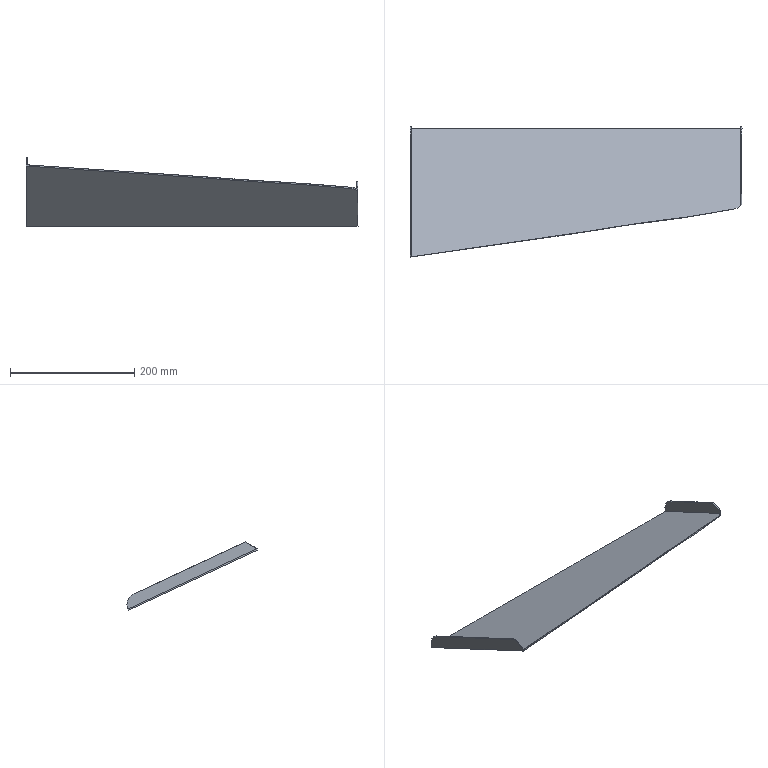Part | NX | features solid 2 | 1 solid | 14 faces | box 535.183 x 209.911 x 110.516 mm | volume 214897 mm3 | plane 9 | spline 3 | cylinder 2 | commonest cylinder face diameters 40 x2
STEP:
#1=CARTESIAN_POINT('',(318.183,710.326,-255.572));
#2=VERTEX_POINT('',#1);
#3=CARTESIAN_POINT('',(318.183,612.464,-209.938));
#4=VERTEX_POINT('',#3);
#5=CARTESIAN_POINT('',(318.183,728.452,-264.024));
#6=DIRECTION('',(0.,-0.9063,0.4226));
#7=VECTOR('',#6,1000.);
#8=LINE('',#5,#7);
#9=EDGE_CURVE('',#2,#4,#8,.T.);
#10=ORIENTED_EDGE('',*,*,#9,.T.);
#11=CARTESIAN_POINT('',(320.183,614.016,-210.661));
#12=VERTEX_POINT('',#11);
#13=CARTESIAN_POINT('',(318.183,612.464,-209.938));
#14=CARTESIAN_POINT('',(318.85,612.981,-210.179));
#15=CARTESIAN_POINT('',(319.516,613.498,-210.42));
#16=CARTESIAN_POINT('',(320.183,614.016,-210.661));
#17=B_SPLINE_CURVE_WITH_KNOTS('',3,(#13,#14,#15,#16),.UNSPECIFIED.,.F.,.F.,(4,4),(0.,1.),.UNSPECIFIED.);
#18=EDGE_CURVE('',#4,#12,#17,.T.);
#19=ORIENTED_EDGE('',*,*,#18,.T.);
#20=CARTESIAN_POINT('',(320.183,710.326,-255.572));
#21=VERTEX_POINT('',#20);
#22=CARTESIAN_POINT('',(320.183,728.452,-264.024));
#23=DIRECTION('',(0.,-0.9063,0.4226));
#24=VECTOR('',#23,1000.);
#25=LINE('',#22,#24);
#26=EDGE_CURVE('',#21,#12,#25,.T.);
#27=ORIENTED_EDGE('',*,*,#26,.F.);
#28=CARTESIAN_POINT('',(214.183,710.326,-255.572));
#29=DIRECTION('',(-1.,0.,0.));
#30=VECTOR('',#29,1000.);
#31=LINE('',#28,#30);
#32=EDGE_CURVE('',#21,#2,#31,.T.);
#33=ORIENTED_EDGE('',*,*,#32,.T.);
#34=EDGE_LOOP('',(#10,#19,#27,#33));
#35=FACE_BOUND('',#34,.T.);
#36=CARTESIAN_POINT('',(214.183,728.452,-264.024));
#37=DIRECTION('',(0.,-0.4226,-0.9063));
#38=DIRECTION('',(0.,-0.9063,0.4226));
#39=AXIS2_PLACEMENT_3D('',#36,#37,#38);
#40=PLANE('',#39);
#41=ADVANCED_FACE('',(#35),#40,.F.);
#42=CARTESIAN_POINT('',(318.183,594.535,-221.438));
#43=VERTEX_POINT('',#42);
#44=CARTESIAN_POINT('',(318.183,594.535,-217.187));
#45=VERTEX_POINT('',#44);
#46=CARTESIAN_POINT('',(318.183,594.535,-221.438));
#47=CARTESIAN_POINT('',(318.183,594.535,-220.021));
#48=CARTESIAN_POINT('',(318.183,594.535,-218.604));
#49=CARTESIAN_POINT('',(318.183,594.535,-217.187));
#50=B_SPLINE_CURVE_WITH_KNOTS('',3,(#46,#47,#48,#49),.UNSPECIFIED.,.F.,.F.,(4,4),(0.,0.00425),.UNSPECIFIED.);
#51=EDGE_CURVE('',#43,#45,#50,.T.);
#52=ORIENTED_EDGE('',*,*,#51,.T.);
#53=CARTESIAN_POINT('',(318.183,594.536,-217.187));
#54=CARTESIAN_POINT('',(318.183,594.907,-217.05));
#55=CARTESIAN_POINT('',(318.183,600.883,-214.633));
#56=CARTESIAN_POINT('',(318.183,612.464,-209.938));
#57=B_SPLINE_CURVE_WITH_KNOTS('',3,(#53,#54,#55,#56),.UNSPECIFIED.,.F.,.F.,(4,4),(0.,1.),.UNSPECIFIED.);
#58=EDGE_CURVE('',#45,#4,#57,.T.);
#59=ORIENTED_EDGE('',*,*,#58,.T.);
#60=ORIENTED_EDGE('',*,*,#9,.F.);
#61=CARTESIAN_POINT('',(318.183,720.,-282.15));
#62=VERTEX_POINT('',#61);
#63=CARTESIAN_POINT('',(318.183,701.874,-273.698));
#64=DIRECTION('',(-1.,0.,0.));
#65=DIRECTION('',(0.,-1.,0.));
#66=AXIS2_PLACEMENT_3D('',#63,#64,#65);
#67=CIRCLE('',#66,20.);
#68=EDGE_CURVE('',#2,#62,#67,.T.);
#69=ORIENTED_EDGE('',*,*,#68,.T.);
#70=CARTESIAN_POINT('',(318.183,720.,-279.943));
#71=VERTEX_POINT('',#70);
#72=CARTESIAN_POINT('',(318.183,720.,-430.));
#73=DIRECTION('',(0.,0.,-1.));
#74=VECTOR('',#73,1000.);
#75=LINE('',#72,#74);
#76=EDGE_CURVE('',#71,#62,#75,.T.);
#77=ORIENTED_EDGE('',*,*,#76,.F.);
#78=CARTESIAN_POINT('',(318.183,417.055,-138.678));
#79=DIRECTION('',(0.,-0.9063,0.4226));
#80=VECTOR('',#79,1000.);
#81=LINE('',#78,#80);
#82=EDGE_CURVE('',#71,#43,#81,.T.);
#83=ORIENTED_EDGE('',*,*,#82,.T.);
#84=EDGE_LOOP('',(#52,#59,#60,#69,#77,#83));
#85=FACE_BOUND('',#84,.T.);
#86=CARTESIAN_POINT('',(318.183,720.,-282.15));
#87=DIRECTION('',(-1.,0.,0.));
#88=DIRECTION('',(0.,-1.,0.));
#89=AXIS2_PLACEMENT_3D('',#86,#87,#88);
#90=PLANE('',#89);
#91=ADVANCED_FACE('',(#85),#90,.T.);
#92=ORIENTED_EDGE('',*,*,#26,.T.);
#93=CARTESIAN_POINT('',(320.183,596.075,-217.946));
#94=VERTEX_POINT('',#93);
#95=CARTESIAN_POINT('',(320.183,614.016,-210.661));
#96=CARTESIAN_POINT('',(320.183,608.036,-213.089));
#97=CARTESIAN_POINT('',(320.183,602.055,-215.518));
#98=CARTESIAN_POINT('',(320.183,596.075,-217.946));
#99=B_SPLINE_CURVE_WITH_KNOTS('',3,(#95,#96,#97,#98),.UNSPECIFIED.,.F.,.F.,(4,4),(0.,1.),.UNSPECIFIED.);
#100=EDGE_CURVE('',#12,#94,#99,.T.);
#101=ORIENTED_EDGE('',*,*,#100,.T.);
#102=CARTESIAN_POINT('',(320.183,596.075,-224.363));
#103=VERTEX_POINT('',#102);
#104=CARTESIAN_POINT('',(320.183,596.075,-217.946));
#105=CARTESIAN_POINT('',(320.183,596.075,-220.085));
#106=CARTESIAN_POINT('',(320.183,596.075,-222.224));
#107=CARTESIAN_POINT('',(320.183,596.075,-224.363));
#108=B_SPLINE_CURVE_WITH_KNOTS('',3,(#104,#105,#106,#107),.UNSPECIFIED.,.F.,.F.,(4,4),(0.01565,0.02207),.UNSPECIFIED.);
#109=EDGE_CURVE('',#94,#103,#108,.T.);
#110=ORIENTED_EDGE('',*,*,#109,.T.);
#111=CARTESIAN_POINT('',(320.183,720.,-282.15));
#112=VERTEX_POINT('',#111);
#113=CARTESIAN_POINT('',(320.183,559.597,-207.353));
#114=DIRECTION('',(0.,-0.9063,0.4226));
#115=VECTOR('',#114,1000.);
#116=LINE('',#113,#115);
#117=EDGE_CURVE('',#112,#103,#116,.T.);
#118=ORIENTED_EDGE('',*,*,#117,.F.);
#119=CARTESIAN_POINT('',(320.183,701.874,-273.698));
#120=DIRECTION('',(1.,0.,0.));
#121=DIRECTION('',(0.,1.,0.));
#122=AXIS2_PLACEMENT_3D('',#119,#120,#121);
#123=CIRCLE('',#122,20.);
#124=EDGE_CURVE('',#112,#21,#123,.T.);
#125=ORIENTED_EDGE('',*,*,#124,.T.);
#126=EDGE_LOOP('',(#92,#101,#110,#118,#125));
#127=FACE_BOUND('',#126,.T.);
#128=CARTESIAN_POINT('',(320.183,560.442,-205.54));
#129=DIRECTION('',(1.,0.,0.));
#130=DIRECTION('',(0.,1.,0.));
#131=AXIS2_PLACEMENT_3D('',#128,#129,#130);
#132=PLANE('',#131);
#133=ADVANCED_FACE('',(#127),#132,.T.);
#134=ORIENTED_EDGE('',*,*,#124,.F.);
#135=CARTESIAN_POINT('',(188.564,720.,-282.15));
#136=DIRECTION('',(-1.,0.,0.));
#137=VECTOR('',#136,1000.);
#138=LINE('',#135,#137);
#139=EDGE_CURVE('',#112,#62,#138,.T.);
#140=ORIENTED_EDGE('',*,*,#139,.T.);
#141=ORIENTED_EDGE('',*,*,#68,.F.);
#142=ORIENTED_EDGE('',*,*,#32,.F.);
#143=EDGE_LOOP('',(#134,#140,#141,#142));
#144=FACE_BOUND('',#143,.T.);
#145=CARTESIAN_POINT('',(214.183,701.874,-273.698));
#146=DIRECTION('',(-1.,0.,0.));
#147=DIRECTION('',(0.,-1.,0.));
#148=AXIS2_PLACEMENT_3D('',#145,#146,#147);
#149=CYLINDRICAL_SURFACE('',#148,20.);
#150=ADVANCED_FACE('',(#144),#149,.T.);
#151=CARTESIAN_POINT('',(-215.,511.962,-185.141));
#152=VERTEX_POINT('',#151);
#153=CARTESIAN_POINT('',(-215.,511.962,-185.141));
#154=CARTESIAN_POINT('',(-192.614,515.2,-186.65));
#155=CARTESIAN_POINT('',(-147.72,520.994,-189.352));
#156=CARTESIAN_POINT('',(-91.827,529.491,-193.314));
#157=CARTESIAN_POINT('',(-47.093,536.174,-196.431));
#158=CARTESIAN_POINT('',(-13.487,540.883,-198.626));
#159=CARTESIAN_POINT('',(20.155,545.387,-200.727));
#160=CARTESIAN_POINT('',(53.73,550.263,-203.001));
#161=CARTESIAN_POINT('',(87.223,555.602,-205.49));
#162=CARTESIAN_POINT('',(120.631,561.41,-208.199));
#163=CARTESIAN_POINT('',(154.136,566.675,-210.654));
#164=CARTESIAN_POINT('',(187.857,570.656,-212.51));
#165=CARTESIAN_POINT('',(215.974,573.885,-214.016));
#166=CARTESIAN_POINT('',(238.337,577.235,-215.578));
#167=CARTESIAN_POINT('',(252.257,579.669,-216.713));
#168=CARTESIAN_POINT('',(263.371,581.734,-217.675));
#169=CARTESIAN_POINT('',(271.697,583.319,-218.415));
#170=CARTESIAN_POINT('',(280.025,584.904,-219.154));
#171=CARTESIAN_POINT('',(288.36,586.451,-219.875));
#172=CARTESIAN_POINT('',(295.322,587.672,-220.445));
#173=CARTESIAN_POINT('',(300.918,588.518,-220.839));
#174=CARTESIAN_POINT('',(305.149,589.032,-221.079));
#175=CARTESIAN_POINT('',(309.34,589.643,-221.364));
#176=CARTESIAN_POINT('',(313.378,591.067,-222.027));
#177=CARTESIAN_POINT('',(316.358,593.032,-222.944));
#178=CARTESIAN_POINT('',(318.506,594.81,-223.773));
#179=CARTESIAN_POINT('',(319.629,595.648,-224.164));
#180=CARTESIAN_POINT('',(320.183,596.075,-224.363));
#181=B_SPLINE_CURVE_WITH_KNOTS('',3,(#153,#154,#155,#156,#157,#158,#159,#160,#161,#162,#163,#164,#165,#166,#167,#168,#169,#170,#171,#172,#173,#174,#175,#176,#177,#178,#179,#180),.UNSPECIFIED.,.F.,.F.,(4,1,1,1,1,1,1,1,1,1,1,1,1,1,1,1,1,1,1,1,1,1,1,1,1,4),(-0.002025,0.06598,0.134,0.168,0.202,0.236,0.27,0.304,0.338,0.372,0.406,0.44,0.457,0.474,0.4825,0.491,0.4995,0.508,0.5165,0.5208,0.525,0.5293,0.5335,0.5378,0.5399,0.542),.UNSPECIFIED.);
#182=EDGE_CURVE('',#152,#103,#181,.T.);
#183=ORIENTED_EDGE('',*,*,#182,.F.);
#184=CARTESIAN_POINT('',(-215.,720.,-282.15));
#185=VERTEX_POINT('',#184);
#186=CARTESIAN_POINT('',(-215.,416.21,-140.491));
#187=DIRECTION('',(0.,0.9063,-0.4226));
#188=VECTOR('',#187,1000.);
#189=LINE('',#186,#188);
#190=EDGE_CURVE('',#152,#185,#189,.T.);
#191=ORIENTED_EDGE('',*,*,#190,.T.);
#192=CARTESIAN_POINT('',(-213.,720.,-282.15));
#193=VERTEX_POINT('',#192);
#194=CARTESIAN_POINT('',(-215.,720.,-282.15));
#195=DIRECTION('',(1.,0.,0.));
#196=VECTOR('',#195,1000.);
#197=LINE('',#194,#196);
#198=EDGE_CURVE('',#185,#193,#197,.T.);
#199=ORIENTED_EDGE('',*,*,#198,.T.);
#200=CARTESIAN_POINT('',(188.564,720.,-282.15));
#201=DIRECTION('',(-1.,0.,0.));
#202=VECTOR('',#201,1000.);
#203=LINE('',#200,#202);
#204=EDGE_CURVE('',#62,#193,#203,.T.);
#205=ORIENTED_EDGE('',*,*,#204,.F.);
#206=ORIENTED_EDGE('',*,*,#139,.F.);
#207=ORIENTED_EDGE('',*,*,#117,.T.);
#208=EDGE_LOOP('',(#183,#191,#199,#205,#206,#207));
#209=FACE_BOUND('',#208,.T.);
#210=CARTESIAN_POINT('',(-353.018,416.21,-140.491));
#211=DIRECTION('',(0.,0.4226,0.9063));
#212=DIRECTION('',(1.,0.,0.));
#213=AXIS2_PLACEMENT_3D('',#210,#211,#212);
#214=PLANE('',#213);
#215=ADVANCED_FACE('',(#209),#214,.F.);
#216=ORIENTED_EDGE('',*,*,#109,.F.);
#217=CARTESIAN_POINT('',(320.183,596.075,-217.946));
#218=CARTESIAN_POINT('',(319.805,595.784,-217.819));
#219=CARTESIAN_POINT('',(319.089,595.237,-217.567));
#220=CARTESIAN_POINT('',(318.515,594.797,-217.314));
#221=CARTESIAN_POINT('',(318.184,594.535,-217.187));
#222=B_SPLINE_CURVE_WITH_KNOTS('',3,(#217,#218,#219,#220,#221),.UNSPECIFIED.,.F.,.F.,(4,1,4),(0.,0.5,1.),.UNSPECIFIED.);
#223=EDGE_CURVE('',#94,#45,#222,.T.);
#224=ORIENTED_EDGE('',*,*,#223,.T.);
#225=ORIENTED_EDGE('',*,*,#51,.F.);
#226=CARTESIAN_POINT('',(310.339,590.055,-219.349));
#227=VERTEX_POINT('',#226);
#228=CARTESIAN_POINT('',(318.183,594.535,-221.438));
#229=CARTESIAN_POINT('',(317.008,593.606,-221.005));
#230=CARTESIAN_POINT('',(314.664,591.763,-220.146));
#231=CARTESIAN_POINT('',(311.819,590.493,-219.553));
#232=CARTESIAN_POINT('',(310.339,590.055,-219.349));
#233=B_SPLINE_CURVE_WITH_KNOTS('',3,(#228,#229,#230,#231,#232),.UNSPECIFIED.,.F.,.F.,(4,1,4),(0.898,0.9027,0.9073),.UNSPECIFIED.);
#234=EDGE_CURVE('',#227,#43,#233,.F.);
#235=ORIENTED_EDGE('',*,*,#234,.F.);
#236=CARTESIAN_POINT('',(-215.,511.962,-183.12));
#237=VERTEX_POINT('',#236);
#238=CARTESIAN_POINT('',(310.339,590.055,-219.349));
#239=CARTESIAN_POINT('',(309.908,589.928,-219.326));
#240=CARTESIAN_POINT('',(308.956,589.678,-219.277));
#241=CARTESIAN_POINT('',(307.478,589.383,-219.201));
#242=CARTESIAN_POINT('',(306.01,589.166,-219.122));
#243=CARTESIAN_POINT('',(304.883,589.012,-219.058));
#244=CARTESIAN_POINT('',(304.15,588.918,-219.016));
#245=CARTESIAN_POINT('',(303.598,588.848,-218.985));
#246=CARTESIAN_POINT('',(303.323,588.814,-218.969));
#247=CARTESIAN_POINT('',(302.88,588.758,-218.942));
#248=CARTESIAN_POINT('',(302.3,588.684,-218.905));
#249=CARTESIAN_POINT('',(301.517,588.58,-218.853));
#250=CARTESIAN_POINT('',(300.667,588.463,-218.795));
#251=CARTESIAN_POINT('',(299.963,588.363,-218.745));
#252=CARTESIAN_POINT('',(299.177,588.249,-218.688));
#253=CARTESIAN_POINT('',(298.555,588.156,-218.642));
#254=CARTESIAN_POINT('',(297.683,588.023,-218.577));
#255=CARTESIAN_POINT('',(296.5,587.838,-218.486));
#256=CARTESIAN_POINT('',(294.913,587.581,-218.36));
#257=CARTESIAN_POINT('',(293.212,587.294,-218.221));
#258=CARTESIAN_POINT('',(291.746,587.04,-218.099));
#259=CARTESIAN_POINT('',(290.942,586.898,-218.031));
#260=CARTESIAN_POINT('',(290.312,586.787,-217.978));
#261=CARTESIAN_POINT('',(290.081,586.746,-217.959));
#262=CARTESIAN_POINT('',(289.638,586.667,-217.921));
#263=CARTESIAN_POINT('',(288.75,586.507,-217.845));
#264=CARTESIAN_POINT('',(287.394,586.262,-217.729));
#265=CARTESIAN_POINT('',(285.072,585.838,-217.528));
#266=CARTESIAN_POINT('',(281.86,585.243,-217.247));
#267=CARTESIAN_POINT('',(276.108,584.161,-216.741));
#268=CARTESIAN_POINT('',(267.427,582.503,-215.966));
#269=CARTESIAN_POINT('',(258.061,580.738,-215.16));
#270=CARTESIAN_POINT('',(249.504,579.191,-214.448));
#271=CARTESIAN_POINT('',(243.121,578.093,-213.939));
#272=CARTESIAN_POINT('',(239.027,577.416,-213.626));
#273=CARTESIAN_POINT('',(236.811,577.058,-213.46));
#274=CARTESIAN_POINT('',(235.444,576.84,-213.36));
#275=CARTESIAN_POINT('',(234.442,576.682,-213.287));
#276=CARTESIAN_POINT('',(233.225,576.492,-213.2));
#277=CARTESIAN_POINT('',(231.088,576.162,-213.049));
#278=CARTESIAN_POINT('',(226.648,575.497,-212.745));
#279=CARTESIAN_POINT('',(221.252,574.737,-212.396));
#280=CARTESIAN_POINT('',(215.531,573.975,-212.045));
#281=CARTESIAN_POINT('',(211.815,573.498,-211.824));
#282=CARTESIAN_POINT('',(208.781,573.117,-211.648));
#283=CARTESIAN_POINT('',(206.813,572.874,-211.535));
#284=CARTESIAN_POINT('',(205.309,572.691,-211.45));
#285=CARTESIAN_POINT('',(203.959,572.527,-211.374));
#286=CARTESIAN_POINT('',(201.526,572.234,-211.237));
#287=CARTESIAN_POINT('',(198.093,571.827,-211.045));
#288=CARTESIAN_POINT('',(193.964,571.345,-210.818));
#289=CARTESIAN_POINT('',(189.847,570.868,-210.593));
#290=CARTESIAN_POINT('',(185.733,570.392,-210.372));
#291=CARTESIAN_POINT('',(182.322,569.996,-210.19));
#292=CARTESIAN_POINT('',(179.914,569.714,-210.063));
#293=CARTESIAN_POINT('',(178.574,569.556,-209.993));
#294=CARTESIAN_POINT('',(177.472,569.426,-209.935));
#295=CARTESIAN_POINT('',(176.742,569.339,-209.897));
#296=CARTESIAN_POINT('',(175.627,569.206,-209.838));
#297=CARTESIAN_POINT('',(173.716,568.977,-209.734));
#298=CARTESIAN_POINT('',(170.89,568.633,-209.576));
#299=CARTESIAN_POINT('',(167.411,568.201,-209.373));
#300=CARTESIAN_POINT('',(162.631,567.594,-209.084));
#301=CARTESIAN_POINT('',(156.403,566.774,-208.689));
#302=CARTESIAN_POINT('',(145.887,565.316,-207.983));
#303=CARTESIAN_POINT('',(134.538,563.592,-207.169));
#304=CARTESIAN_POINT('',(123.85,561.853,-206.359));
#305=CARTESIAN_POINT('',(118.331,560.935,-205.931));
#306=CARTESIAN_POINT('',(115.102,560.394,-205.679));
#307=CARTESIAN_POINT('',(112.711,559.991,-205.49));
#308=CARTESIAN_POINT('',(110.073,559.545,-205.281));
#309=CARTESIAN_POINT('',(106.698,558.973,-205.015));
#310=CARTESIAN_POINT('',(100.867,557.982,-204.557));
#311=CARTESIAN_POINT('',(92.9,556.63,-203.937));
#312=CARTESIAN_POINT('',(83.873,555.122,-203.243));
#313=CARTESIAN_POINT('',(75.395,553.738,-202.599));
#314=CARTESIAN_POINT('',(67.469,552.472,-202.007));
#315=CARTESIAN_POINT('',(61.327,551.511,-201.556));
#316=CARTESIAN_POINT('',(56.697,550.796,-201.221));
#317=CARTESIAN_POINT('',(53.358,550.285,-200.982));
#318=CARTESIAN_POINT('',(50.713,549.884,-200.795));
#319=CARTESIAN_POINT('',(48.623,549.569,-200.649));
#320=CARTESIAN_POINT('',(47.211,549.357,-200.55));
#321=CARTESIAN_POINT('',(45.378,549.083,-200.424));
#322=CARTESIAN_POINT('',(43.013,548.731,-200.261));
#323=CARTESIAN_POINT('',(38.67,548.09,-199.965));
#324=CARTESIAN_POINT('',(33.409,547.325,-199.613));
#325=CARTESIAN_POINT('',(27.818,546.527,-199.244));
#326=CARTESIAN_POINT('',(23.462,545.912,-198.959));
#327=CARTESIAN_POINT('',(19.707,545.387,-198.715));
#328=CARTESIAN_POINT('',(16.991,545.011,-198.539));
#329=CARTESIAN_POINT('',(15.446,544.797,-198.44));
#330=CARTESIAN_POINT('',(14.202,544.625,-198.36));
#331=CARTESIAN_POINT('',(13.234,544.492,-198.298));
#332=CARTESIAN_POINT('',(11.846,544.301,-198.209));
#333=CARTESIAN_POINT('',(9.463,543.974,-198.056));
#334=CARTESIAN_POINT('',(4.666,543.318,-197.749));
#335=CARTESIAN_POINT('',(-0.8003,542.575,-197.399));
#336=CARTESIAN_POINT('',(-6.269,541.832,-197.051));
#337=CARTESIAN_POINT('',(-9.685,541.367,-196.833));
#338=CARTESIAN_POINT('',(-12.417,540.994,-196.659));
#339=CARTESIAN_POINT('',(-14.468,540.714,-196.529));
#340=CARTESIAN_POINT('',(-16.169,540.481,-196.421));
#341=CARTESIAN_POINT('',(-17.375,540.316,-196.344));
#342=CARTESIAN_POINT('',(-18.04,540.224,-196.302));
#343=CARTESIAN_POINT('',(-18.605,540.147,-196.266));
#344=CARTESIAN_POINT('',(-18.919,540.104,-196.246));
#345=CARTESIAN_POINT('',(-19.428,540.034,-196.214));
#346=CARTESIAN_POINT('',(-20.286,539.916,-196.159));
#347=CARTESIAN_POINT('',(-21.557,539.74,-196.078));
#348=CARTESIAN_POINT('',(-23.108,539.526,-195.978));
#349=CARTESIAN_POINT('',(-25.228,539.232,-195.841));
#350=CARTESIAN_POINT('',(-27.968,538.851,-195.663));
#351=CARTESIAN_POINT('',(-32.543,538.209,-195.362));
#352=CARTESIAN_POINT('',(-38.623,537.346,-194.957));
#353=CARTESIAN_POINT('',(-49.124,535.833,-194.249));
#354=CARTESIAN_POINT('',(-60.768,534.123,-193.449));
#355=CARTESIAN_POINT('',(-73.611,532.208,-192.556));
#356=CARTESIAN_POINT('',(-82.05,530.942,-191.965));
#357=CARTESIAN_POINT('',(-89.269,529.855,-191.458));
#358=CARTESIAN_POINT('',(-96.132,528.821,-190.978));
#359=CARTESIAN_POINT('',(-104.35,527.585,-190.406));
#360=CARTESIAN_POINT('',(-113.537,526.21,-189.77));
#361=CARTESIAN_POINT('',(-122.071,524.944,-189.183));
#362=CARTESIAN_POINT('',(-129.945,523.79,-188.646));
#363=CARTESIAN_POINT('',(-135.957,522.92,-188.24));
#364=CARTESIAN_POINT('',(-140.436,522.28,-187.94));
#365=CARTESIAN_POINT('',(-143.628,521.826,-187.728));
#366=CARTESIAN_POINT('',(-146.156,521.47,-187.561));
#367=CARTESIAN_POINT('',(-147.843,521.234,-187.45));
#368=CARTESIAN_POINT('',(-148.683,521.117,-187.395));
#369=CARTESIAN_POINT('',(-149.133,521.054,-187.366));
#370=CARTESIAN_POINT('',(-149.537,520.997,-187.339));
#371=CARTESIAN_POINT('',(-149.677,520.978,-187.33));
#372=CARTESIAN_POINT('',(-149.971,520.937,-187.311));
#373=CARTESIAN_POINT('',(-150.478,520.866,-187.278));
#374=CARTESIAN_POINT('',(-151.325,520.749,-187.223));
#375=CARTESIAN_POINT('',(-152.492,520.587,-187.148));
#376=CARTESIAN_POINT('',(-154.266,520.341,-187.034));
#377=CARTESIAN_POINT('',(-156.884,519.98,-186.867));
#378=CARTESIAN_POINT('',(-160.669,519.46,-186.626));
#379=CARTESIAN_POINT('',(-165.096,518.856,-186.344));
#380=CARTESIAN_POINT('',(-169.32,518.281,-186.076));
#381=CARTESIAN_POINT('',(-173.018,517.78,-185.841));
#382=CARTESIAN_POINT('',(-175.956,517.381,-185.655));
#383=CARTESIAN_POINT('',(-178.524,517.033,-185.492));
#384=CARTESIAN_POINT('',(-180.417,516.776,-185.373));
#385=CARTESIAN_POINT('',(-181.48,516.631,-185.305));
#386=CARTESIAN_POINT('',(-182.397,516.507,-185.247));
#387=CARTESIAN_POINT('',(-182.903,516.438,-185.215));
#388=CARTESIAN_POINT('',(-183.717,516.327,-185.163));
#389=CARTESIAN_POINT('',(-185.065,516.143,-185.078));
#390=CARTESIAN_POINT('',(-187.001,515.88,-184.955));
#391=CARTESIAN_POINT('',(-189.268,515.57,-184.81));
#392=CARTESIAN_POINT('',(-192.239,515.163,-184.619));
#393=CARTESIAN_POINT('',(-195.849,514.666,-184.386));
#394=CARTESIAN_POINT('',(-201.404,513.895,-184.025));
#395=CARTESIAN_POINT('',(-207.934,512.978,-183.595));
#396=CARTESIAN_POINT('',(-212.718,512.292,-183.274));
#397=CARTESIAN_POINT('',(-215.,511.962,-183.12));
#398=B_SPLINE_CURVE_WITH_KNOTS('',3,(#238,#239,#240,#241,#242,#243,#244,#245,#246,#247,#248,#249,#250,#251,#252,#253,#254,#255,#256,#257,#258,#259,#260,#261,#262,#263,#264,#265,#266,#267,#268,#269,#270,#271,#272,#273,#274,#275,#276,#277,#278,#279,#280,#281,#282,#283,#284,#285,#286,#287,#288,#289,#290,#291,#292,#293,#294,#295,#296,#297,#298,#299,#300,#301,#302,#303,#304,#305,#306,#307,#308,#309,#310,#311,#312,#313,#314,#315,#316,#317,#318,#319,#320,#321,#322,#323,#324,#325,#326,#327,#328,#329,#330,#331,#332,#333,#334,#335,#336,#337,#338,#339,#340,#341,#342,#343,#344,#345,#346,#347,#348,#349,#350,#351,#352,#353,#354,#355,#356,#357,#358,#359,#360,#361,#362,#363,#364,#365,#366,#367,#368,#369,#370,#371,#372,#373,#374,#375,#376,#377,#378,#379,#380,#381,#382,#383,#384,#385,#386,#387,#388,#389,#390,#391,#392,#393,#394,#395,#396,#397),.UNSPECIFIED.,.F.,.F.,(4,1,1,1,1,1,1,1,1,1,1,1,1,1,1,1,1,1,1,1,1,1,1,1,1,1,1,1,1,1,1,1,1,1,1,1,1,1,1,1,1,1,1,1,1,1,1,1,1,1,1,1,1,1,1,1,1,1,1,1,1,1,1,1,1,1,1,1,1,1,1,1,1,1,1,1,1,1,1,1,1,1,1,1,1,1,1,1,1,1,1,1,1,1,1,1,1,1,1,1,1,1,1,1,1,1,1,1,1,1,1,1,1,1,1,1,1,1,1,1,1,1,1,1,1,1,1,1,1,1,1,1,1,1,1,1,1,1,1,1,1,1,1,1,1,1,1,1,1,1,1,1,1,1,1,1,1,4),(0.,0.001953,0.003906,0.005859,0.007812,0.008301,0.008789,0.009766,0.01074,0.01172,0.01367,0.01562,0.0166,0.01758,0.01953,0.02148,0.02344,0.02734,0.03125,0.0332,0.03516,0.03564,0.03613,0.03711,0.03906,0.04297,0.04688,0.05469,0.0625,0.07812,0.09375,0.1094,0.125,0.1328,0.1367,0.1406,0.1426,0.1445,0.1484,0.1562,0.1719,0.1797,0.1875,0.1914,0.1953,0.1973,0.1992,0.2031,0.2109,0.2188,0.2266,0.2344,0.2422,0.2461,0.248,0.25,0.252,0.2539,0.2578,0.2656,0.2734,0.2812,0.2969,0.3125,0.3438,0.3594,0.3672,0.3711,0.375,0.3789,0.3828,0.3906,0.4062,0.4219,0.4375,0.4531,0.4688,0.4766,0.4844,0.4922,0.4961,0.5,0.5039,0.5078,0.5156,0.5312,0.5391,0.5469,0.5547,0.5586,0.5605,0.5625,0.5645,0.5664,0.5703,0.5781,0.5938,0.6016,0.6094,0.6133,0.6172,0.6211,0.623,0.624,0.625,0.626,0.627,0.6289,0.6328,0.6367,0.6406,0.6484,0.6562,0.6719,0.6875,0.7188,0.7344,0.75,0.7578,0.7656,0.7812,0.7969,0.8125,0.8281,0.8438,0.8516,0.8594,0.8672,0.8711,0.873,0.874,0.875,0.876,0.877,0.8789,0.8828,0.8867,0.8906,0.8984,0.9062,0.9141,0.9219,0.9258,0.9297,0.9336,0.9355,0.9365,0.9375,0.9385,0.9395,0.9414,0.9453,0.9492,0.9531,0.9609,0.9688,0.9844,1.),.UNSPECIFIED.);
#399=EDGE_CURVE('',#227,#237,#398,.T.);
#400=ORIENTED_EDGE('',*,*,#399,.T.);
#401=CARTESIAN_POINT('',(-215.,511.962,-169.07));
#402=DIRECTION('',(0.,0.,1.));
#403=VECTOR('',#402,1000.);
#404=LINE('',#401,#403);
#405=EDGE_CURVE('',#152,#237,#404,.T.);
#406=ORIENTED_EDGE('',*,*,#405,.F.);
#407=ORIENTED_EDGE('',*,*,#182,.T.);
#408=EDGE_LOOP('',(#216,#224,#225,#235,#400,#406,#407));
#409=FACE_BOUND('',#408,.T.);
#410=CARTESIAN_POINT('',(322.97,598.236,-224.61));
#411=CARTESIAN_POINT('',(322.97,598.236,-182.872));
#412=CARTESIAN_POINT('',(322.36,597.762,-224.61));
#413=CARTESIAN_POINT('',(322.36,597.762,-182.872));
#414=CARTESIAN_POINT('',(321.144,596.817,-224.61));
#415=CARTESIAN_POINT('',(321.144,596.817,-182.872));
#416=CARTESIAN_POINT('',(319.286,595.382,-224.61));
#417=CARTESIAN_POINT('',(319.286,595.382,-182.872));
#418=CARTESIAN_POINT('',(318.053,594.458,-224.61));
#419=CARTESIAN_POINT('',(318.053,594.458,-182.872));
#420=CARTESIAN_POINT('',(315.837,592.59,-224.61));
#421=CARTESIAN_POINT('',(315.837,592.59,-182.872));
#422=CARTESIAN_POINT('',(312.253,590.601,-224.61));
#423=CARTESIAN_POINT('',(312.253,590.601,-182.872));
#424=CARTESIAN_POINT('',(309.557,589.816,-224.61));
#425=CARTESIAN_POINT('',(309.557,589.816,-182.872));
#426=CARTESIAN_POINT('',(307.306,589.332,-224.61));
#427=CARTESIAN_POINT('',(307.306,589.332,-182.872));
#428=CARTESIAN_POINT('',(305.204,589.056,-224.61));
#429=CARTESIAN_POINT('',(305.204,589.056,-182.872));
#430=CARTESIAN_POINT('',(303.109,588.787,-224.61));
#431=CARTESIAN_POINT('',(303.109,588.787,-182.872));
#432=CARTESIAN_POINT('',(301.098,588.527,-224.61));
#433=CARTESIAN_POINT('',(301.098,588.527,-182.872));
#434=CARTESIAN_POINT('',(298.403,588.14,-224.61));
#435=CARTESIAN_POINT('',(298.403,588.14,-182.872));
#436=CARTESIAN_POINT('',(295.054,587.612,-224.61));
#437=CARTESIAN_POINT('',(295.054,587.612,-182.872));
#438=CARTESIAN_POINT('',(291.029,586.919,-224.61));
#439=CARTESIAN_POINT('',(291.029,586.919,-182.872));
#440=CARTESIAN_POINT('',(286.979,586.189,-224.61));
#441=CARTESIAN_POINT('',(286.979,586.189,-182.872));
#442=CARTESIAN_POINT('',(282.892,585.436,-224.61));
#443=CARTESIAN_POINT('',(282.892,585.436,-182.872));
#444=CARTESIAN_POINT('',(277.404,584.406,-224.61));
#445=CARTESIAN_POINT('',(277.404,584.406,-182.872));
#446=CARTESIAN_POINT('',(270.479,583.087,-224.61));
#447=CARTESIAN_POINT('',(270.479,583.087,-182.872));
#448=CARTESIAN_POINT('',(262.104,581.495,-224.61));
#449=CARTESIAN_POINT('',(262.104,581.495,-182.872));
#450=CARTESIAN_POINT('',(250.902,579.425,-224.61));
#451=CARTESIAN_POINT('',(250.902,579.425,-182.872));
#452=CARTESIAN_POINT('',(236.854,576.991,-224.61));
#453=CARTESIAN_POINT('',(236.854,576.991,-182.872));
#454=CARTESIAN_POINT('',(219.909,574.5,-224.61));
#455=CARTESIAN_POINT('',(219.909,574.5,-182.872));
#456=CARTESIAN_POINT('',(202.958,572.376,-224.61));
#457=CARTESIAN_POINT('',(202.958,572.376,-182.872));
#458=CARTESIAN_POINT('',(180.52,569.805,-224.61));
#459=CARTESIAN_POINT('',(180.52,569.805,-182.872));
#460=CARTESIAN_POINT('',(152.805,566.485,-224.61));
#461=CARTESIAN_POINT('',(152.805,566.485,-182.872));
#462=CARTESIAN_POINT('',(119.67,561.243,-224.61));
#463=CARTESIAN_POINT('',(119.67,561.243,-182.872));
#464=CARTESIAN_POINT('',(86.394,555.463,-224.61));
#465=CARTESIAN_POINT('',(86.394,555.463,-182.872));
#466=CARTESIAN_POINT('',(52.853,550.129,-224.61));
#467=CARTESIAN_POINT('',(52.853,550.129,-182.872));
#468=CARTESIAN_POINT('',(19.243,545.262,-224.61));
#469=CARTESIAN_POINT('',(19.243,545.262,-182.872));
#470=CARTESIAN_POINT('',(-14.288,540.775,-224.61));
#471=CARTESIAN_POINT('',(-14.288,540.775,-182.872));
#472=CARTESIAN_POINT('',(-47.714,536.083,-224.61));
#473=CARTESIAN_POINT('',(-47.714,536.083,-182.872));
#474=CARTESIAN_POINT('',(-92.202,529.433,-224.61));
#475=CARTESIAN_POINT('',(-92.202,529.433,-182.872));
#476=CARTESIAN_POINT('',(-148.053,520.95,-224.61));
#477=CARTESIAN_POINT('',(-148.053,520.95,-182.872));
#478=CARTESIAN_POINT('',(-192.78,515.176,-224.61));
#479=CARTESIAN_POINT('',(-192.78,515.176,-182.872));
#480=CARTESIAN_POINT('',(-215.,511.962,-224.61));
#481=CARTESIAN_POINT('',(-215.,511.962,-182.872));
#482=B_SPLINE_SURFACE_WITH_KNOTS('',3,1,((#410,#411),(#412,#413),(#414,#415),(#416,#417),(#418,#419),(#420,#421),(#422,#423),(#424,#425),(#426,#427),(#428,#429),(#430,#431),(#432,#433),(#434,#435),(#436,#437),(#438,#439),(#440,#441),(#442,#443),(#444,#445),(#446,#447),(#448,#449),(#450,#451),(#452,#453),(#454,#455),(#456,#457),(#458,#459),(#460,#461),(#462,#463),(#464,#465),(#466,#467),(#468,#469),(#470,#471),(#472,#473),(#474,#475),(#476,#477),(#478,#479),(#480,#481)),.SURF_OF_LINEAR_EXTRUSION.,.F.,.F.,.F.,(4,1,1,1,1,1,1,1,1,1,1,1,1,1,1,1,1,1,1,1,1,1,1,1,1,1,1,1,1,1,1,1,1,4),(2,2),(-0.002007,-0.000379,0.001249,0.002877,0.004504,0.006132,0.006946,0.00776,0.009388,0.01102,0.01264,0.01427,0.01753,0.02078,0.02404,0.02729,0.03055,0.03706,0.04357,0.05008,0.0631,0.07613,0.08915,0.1022,0.1282,0.1543,0.1803,0.2063,0.2324,0.2584,0.2845,0.3105,0.3626,0.4147),(0.,1.),.UNSPECIFIED.);
#483=ADVANCED_FACE('',(#409),#482,.F.);
#484=CARTESIAN_POINT('',(-213.,512.424,-183.149));
#485=VERTEX_POINT('',#484);
#486=CARTESIAN_POINT('',(-213.,720.,-279.943));
#487=VERTEX_POINT('',#486);
#488=CARTESIAN_POINT('',(-213.,417.055,-138.678));
#489=DIRECTION('',(0.,0.9063,-0.4226));
#490=VECTOR('',#489,1000.);
#491=LINE('',#488,#490);
#492=EDGE_CURVE('',#485,#487,#491,.T.);
#493=ORIENTED_EDGE('',*,*,#492,.F.);
#494=CARTESIAN_POINT('',(-213.,512.424,-183.149));
#495=CARTESIAN_POINT('',(-210.745,512.749,-183.301));
#496=CARTESIAN_POINT('',(-205.996,513.427,-183.617));
#497=CARTESIAN_POINT('',(-199.466,514.343,-184.044));
#498=CARTESIAN_POINT('',(-193.887,515.116,-184.404));
#499=CARTESIAN_POINT('',(-189.522,515.717,-184.685));
#500=CARTESIAN_POINT('',(-185.745,516.233,-184.925));
#501=CARTESIAN_POINT('',(-183.005,516.606,-185.099));
#502=CARTESIAN_POINT('',(-181.445,516.818,-185.198));
#503=CARTESIAN_POINT('',(-180.183,516.989,-185.278));
#504=CARTESIAN_POINT('',(-179.222,517.119,-185.338));
#505=CARTESIAN_POINT('',(-177.835,517.307,-185.426));
#506=CARTESIAN_POINT('',(-175.457,517.629,-185.576));
#507=CARTESIAN_POINT('',(-172.036,518.092,-185.792));
#508=CARTESIAN_POINT('',(-168.618,518.554,-186.007));
#509=CARTESIAN_POINT('',(-166.235,518.876,-186.158));
#510=CARTESIAN_POINT('',(-165.029,519.038,-186.233));
#511=CARTESIAN_POINT('',(-164.362,519.128,-186.275));
#512=CARTESIAN_POINT('',(-163.799,519.204,-186.311));
#513=CARTESIAN_POINT('',(-163.477,519.248,-186.331));
#514=CARTESIAN_POINT('',(-162.949,519.319,-186.365));
#515=CARTESIAN_POINT('',(-162.034,519.444,-186.422));
#516=CARTESIAN_POINT('',(-160.051,519.715,-186.549));
#517=CARTESIAN_POINT('',(-157.513,520.065,-186.712));
#518=CARTESIAN_POINT('',(-154.688,520.458,-186.895));
#519=CARTESIAN_POINT('',(-152.425,520.774,-187.043));
#520=CARTESIAN_POINT('',(-150.43,521.053,-187.173));
#521=CARTESIAN_POINT('',(-148.954,521.261,-187.27));
#522=CARTESIAN_POINT('',(-148.119,521.378,-187.324));
#523=CARTESIAN_POINT('',(-147.409,521.478,-187.371));
#524=CARTESIAN_POINT('',(-146.978,521.539,-187.399));
#525=CARTESIAN_POINT('',(-146.304,521.634,-187.444));
#526=CARTESIAN_POINT('',(-145.168,521.794,-187.518));
#527=CARTESIAN_POINT('',(-143.515,522.028,-187.628));
#528=CARTESIAN_POINT('',(-141.531,522.31,-187.759));
#529=CARTESIAN_POINT('',(-138.867,522.689,-187.936));
#530=CARTESIAN_POINT('',(-135.512,523.17,-188.16));
#531=CARTESIAN_POINT('',(-131.442,523.756,-188.433));
#532=CARTESIAN_POINT('',(-127.328,524.353,-188.712));
#533=CARTESIAN_POINT('',(-123.864,524.858,-188.947));
#534=CARTESIAN_POINT('',(-121.071,525.267,-189.138));
#535=CARTESIAN_POINT('',(-119.316,525.525,-189.258));
#536=CARTESIAN_POINT('',(-117.908,525.733,-189.355));
#537=CARTESIAN_POINT('',(-116.846,525.889,-189.428));
#538=CARTESIAN_POINT('',(-115.969,526.019,-189.489));
#539=CARTESIAN_POINT('',(-115.333,526.113,-189.532));
#540=CARTESIAN_POINT('',(-115.003,526.162,-189.555));
#541=CARTESIAN_POINT('',(-114.661,526.212,-189.579));
#542=CARTESIAN_POINT('',(-114.676,526.21,-189.578));
#543=CARTESIAN_POINT('',(-114.566,526.227,-189.585));
#544=CARTESIAN_POINT('',(-114.421,526.248,-189.595));
#545=CARTESIAN_POINT('',(-114.152,526.288,-189.614));
#546=CARTESIAN_POINT('',(-113.795,526.341,-189.639));
#547=CARTESIAN_POINT('',(-113.248,526.423,-189.677));
#548=CARTESIAN_POINT('',(-112.443,526.543,-189.733));
#549=CARTESIAN_POINT('',(-110.894,526.775,-189.841));
#550=CARTESIAN_POINT('',(-108.467,527.139,-190.011));
#551=CARTESIAN_POINT('',(-104.771,527.694,-190.269));
#552=CARTESIAN_POINT('',(-100.291,528.366,-190.583));
#553=CARTESIAN_POINT('',(-95.904,529.026,-190.891));
#554=CARTESIAN_POINT('',(-92.003,529.612,-191.164));
#555=CARTESIAN_POINT('',(-89.401,530.004,-191.347));
#556=CARTESIAN_POINT('',(-87.223,530.331,-191.499));
#557=CARTESIAN_POINT('',(-85.537,530.585,-191.618));
#558=CARTESIAN_POINT('',(-84.1,530.801,-191.719));
#559=CARTESIAN_POINT('',(-83.057,530.958,-191.792));
#560=CARTESIAN_POINT('',(-82.479,531.045,-191.832));
#561=CARTESIAN_POINT('',(-81.973,531.121,-191.868));
#562=CARTESIAN_POINT('',(-81.729,531.158,-191.885));
#563=CARTESIAN_POINT('',(-81.313,531.22,-191.914));
#564=CARTESIAN_POINT('',(-80.63,531.323,-191.962));
#565=CARTESIAN_POINT('',(-79.639,531.472,-192.031));
#566=CARTESIAN_POINT('',(-78.471,531.648,-192.113));
#567=CARTESIAN_POINT('',(-76.924,531.88,-192.221));
#568=CARTESIAN_POINT('',(-75.019,532.165,-192.355));
#569=CARTESIAN_POINT('',(-72.029,532.613,-192.563));
#570=CARTESIAN_POINT('',(-68.402,533.154,-192.816));
#571=CARTESIAN_POINT('',(-64.225,533.776,-193.105));
#572=CARTESIAN_POINT('',(-60.223,534.368,-193.382));
#573=CARTESIAN_POINT('',(-56.399,534.933,-193.645));
#574=CARTESIAN_POINT('',(-53.352,535.38,-193.854));
#575=CARTESIAN_POINT('',(-51.311,535.679,-193.993));
#576=CARTESIAN_POINT('',(-50.143,535.849,-194.072));
#577=CARTESIAN_POINT('',(-49.343,535.966,-194.127));
#578=CARTESIAN_POINT('',(-48.305,536.117,-194.197));
#579=CARTESIAN_POINT('',(-47.,536.307,-194.286));
#580=CARTESIAN_POINT('',(-44.671,536.644,-194.443));
#581=CARTESIAN_POINT('',(-40.006,537.316,-194.756));
#582=CARTESIAN_POINT('',(-33.242,538.279,-195.206));
#583=CARTESIAN_POINT('',(-26.35,539.247,-195.657));
#584=CARTESIAN_POINT('',(-20.789,540.02,-196.017));
#585=CARTESIAN_POINT('',(-16.513,540.609,-196.292));
#586=CARTESIAN_POINT('',(-12.464,541.165,-196.551));
#587=CARTESIAN_POINT('',(-6.985,541.917,-196.902));
#588=CARTESIAN_POINT('',(2.554,543.225,-197.512));
#589=CARTESIAN_POINT('',(13.558,544.723,-198.21));
#590=CARTESIAN_POINT('',(24.316,546.204,-198.901));
#591=CARTESIAN_POINT('',(32.482,547.362,-199.441));
#592=CARTESIAN_POINT('',(39.331,548.354,-199.904));
#593=CARTESIAN_POINT('',(44.815,549.163,-200.281));
#594=CARTESIAN_POINT('',(49.006,549.789,-200.572));
#595=CARTESIAN_POINT('',(52.959,550.385,-200.851));
#596=CARTESIAN_POINT('',(57.004,551.002,-201.138));
#597=CARTESIAN_POINT('',(61.05,551.627,-201.43));
#598=CARTESIAN_POINT('',(65.123,552.263,-201.726));
#599=CARTESIAN_POINT('',(69.215,552.909,-202.027));
#600=CARTESIAN_POINT('',(73.331,553.565,-202.334));
#601=CARTESIAN_POINT('',(76.77,554.12,-202.592));
#602=CARTESIAN_POINT('',(79.204,554.515,-202.776));
#603=CARTESIAN_POINT('',(80.571,554.738,-202.88));
#604=CARTESIAN_POINT('',(81.672,554.918,-202.964));
#605=CARTESIAN_POINT('',(82.488,555.052,-203.027));
#606=CARTESIAN_POINT('',(83.707,555.252,-203.12));
#607=CARTESIAN_POINT('',(85.856,555.606,-203.285));
#608=CARTESIAN_POINT('',(89.138,556.151,-203.539));
#609=CARTESIAN_POINT('',(92.648,556.739,-203.813));
#610=CARTESIAN_POINT('',(95.252,557.177,-204.018));
#611=CARTESIAN_POINT('',(96.753,557.43,-204.136));
#612=CARTESIAN_POINT('',(97.966,557.635,-204.231));
#613=CARTESIAN_POINT('',(98.932,557.798,-204.307));
#614=CARTESIAN_POINT('',(100.307,558.03,-204.416));
#615=CARTESIAN_POINT('',(102.672,558.431,-204.602));
#616=CARTESIAN_POINT('',(106.076,559.007,-204.871));
#617=CARTESIAN_POINT('',(109.453,559.58,-205.138));
#618=CARTESIAN_POINT('',(112.2,560.047,-205.356));
#619=CARTESIAN_POINT('',(114.142,560.377,-205.51));
#620=CARTESIAN_POINT('',(116.532,560.783,-205.699));
#621=CARTESIAN_POINT('',(119.507,561.283,-205.933));
#622=CARTESIAN_POINT('',(124.674,562.143,-206.334));
#623=CARTESIAN_POINT('',(131.687,563.282,-206.865));
#624=CARTESIAN_POINT('',(138.261,564.31,-207.344));
#625=CARTESIAN_POINT('',(143.277,565.069,-207.698));
#626=CARTESIAN_POINT('',(148.026,565.771,-208.025));
#627=CARTESIAN_POINT('',(154.275,566.657,-208.438));
#628=CARTESIAN_POINT('',(160.911,567.545,-208.853));
#629=CARTESIAN_POINT('',(166.459,568.26,-209.186));
#630=CARTESIAN_POINT('',(170.733,568.797,-209.436));
#631=CARTESIAN_POINT('',(174.411,569.248,-209.646));
#632=CARTESIAN_POINT('',(177.372,569.604,-209.813));
#633=CARTESIAN_POINT('',(179.732,569.885,-209.944));
#634=CARTESIAN_POINT('',(181.705,570.117,-210.052));
#635=CARTESIAN_POINT('',(184.471,570.442,-210.203));
#636=CARTESIAN_POINT('',(187.885,570.838,-210.388));
#637=CARTESIAN_POINT('',(191.309,571.231,-210.571));
#638=CARTESIAN_POINT('',(193.718,571.505,-210.699));
#639=CARTESIAN_POINT('',(195.071,571.658,-210.77));
#640=CARTESIAN_POINT('',(196.152,571.779,-210.827));
#641=CARTESIAN_POINT('',(196.979,571.873,-210.871));
#642=CARTESIAN_POINT('',(198.202,572.013,-210.936));
#643=CARTESIAN_POINT('',(200.364,572.264,-211.053));
#644=CARTESIAN_POINT('',(203.664,572.658,-211.237));
#645=CARTESIAN_POINT('',(207.219,573.095,-211.441));
#646=CARTESIAN_POINT('',(210.196,573.469,-211.615));
#647=CARTESIAN_POINT('',(213.35,573.869,-211.801));
#648=CARTESIAN_POINT('',(216.936,574.335,-212.018));
#649=CARTESIAN_POINT('',(221.145,574.899,-212.282));
#650=CARTESIAN_POINT('',(225.163,575.459,-212.543));
#651=CARTESIAN_POINT('',(228.896,575.997,-212.794));
#652=CARTESIAN_POINT('',(232.816,576.587,-213.069));
#653=CARTESIAN_POINT('',(236.837,577.218,-213.363));
#654=CARTESIAN_POINT('',(240.282,577.778,-213.624));
#655=CARTESIAN_POINT('',(242.76,578.191,-213.817));
#656=CARTESIAN_POINT('',(244.166,578.428,-213.927));
#657=CARTESIAN_POINT('',(245.296,578.621,-214.017));
#658=CARTESIAN_POINT('',(246.172,578.771,-214.087));
#659=CARTESIAN_POINT('',(247.447,578.99,-214.189));
#660=CARTESIAN_POINT('',(249.674,579.378,-214.37));
#661=CARTESIAN_POINT('',(252.33,579.848,-214.59));
#662=CARTESIAN_POINT('',(255.069,580.341,-214.82));
#663=CARTESIAN_POINT('',(256.821,580.66,-214.968));
#664=CARTESIAN_POINT('',(258.243,580.92,-215.089));
#665=CARTESIAN_POINT('',(259.325,581.119,-215.182));
#666=CARTESIAN_POINT('',(260.223,581.285,-215.26));
#667=CARTESIAN_POINT('',(260.883,581.408,-215.317));
#668=CARTESIAN_POINT('',(261.219,581.47,-215.346));
#669=CARTESIAN_POINT('',(261.593,581.539,-215.378));
#670=CARTESIAN_POINT('',(261.504,581.523,-215.37));
#671=CARTESIAN_POINT('',(261.561,581.533,-215.375));
#672=CARTESIAN_POINT('',(261.594,581.54,-215.378));
#673=CARTESIAN_POINT('',(261.689,581.558,-215.387));
#674=CARTESIAN_POINT('',(261.849,581.588,-215.401));
#675=CARTESIAN_POINT('',(262.128,581.641,-215.425));
#676=CARTESIAN_POINT('',(262.738,581.756,-215.479));
#677=CARTESIAN_POINT('',(263.811,581.959,-215.574));
#678=CARTESIAN_POINT('',(265.592,582.297,-215.731));
#679=CARTESIAN_POINT('',(267.868,582.728,-215.932));
#680=CARTESIAN_POINT('',(270.176,583.165,-216.136));
#681=CARTESIAN_POINT('',(272.269,583.562,-216.321));
#682=CARTESIAN_POINT('',(273.966,583.883,-216.471));
#683=CARTESIAN_POINT('',(275.473,584.169,-216.604));
#684=CARTESIAN_POINT('',(276.6,584.382,-216.704));
#685=CARTESIAN_POINT('',(277.232,584.502,-216.76));
#686=CARTESIAN_POINT('',(277.791,584.608,-216.809));
#687=CARTESIAN_POINT('',(278.061,584.659,-216.833));
#688=CARTESIAN_POINT('',(278.518,584.745,-216.873));
#689=CARTESIAN_POINT('',(279.262,584.886,-216.939));
#690=CARTESIAN_POINT('',(280.326,585.086,-217.032));
#691=CARTESIAN_POINT('',(281.553,585.317,-217.14));
#692=CARTESIAN_POINT('',(283.14,585.614,-217.278));
#693=CARTESIAN_POINT('',(285.027,585.965,-217.442));
#694=CARTESIAN_POINT('',(287.135,586.353,-217.623));
#695=CARTESIAN_POINT('',(289.09,586.709,-217.789));
#696=CARTESIAN_POINT('',(290.885,587.031,-217.939));
#697=CARTESIAN_POINT('',(292.264,587.275,-218.053));
#698=CARTESIAN_POINT('',(293.138,587.427,-218.124));
#699=CARTESIAN_POINT('',(293.653,587.516,-218.165));
#700=CARTESIAN_POINT('',(293.932,587.564,-218.188));
#701=CARTESIAN_POINT('',(294.576,587.674,-218.239));
#702=CARTESIAN_POINT('',(295.295,587.795,-218.295));
#703=CARTESIAN_POINT('',(296.589,588.01,-218.395));
#704=CARTESIAN_POINT('',(298.33,588.287,-218.525));
#705=CARTESIAN_POINT('',(299.99,588.538,-218.641));
#706=CARTESIAN_POINT('',(301.243,588.717,-218.725));
#707=CARTESIAN_POINT('',(302.191,588.848,-218.786));
#708=CARTESIAN_POINT('',(302.836,588.932,-218.825));
#709=CARTESIAN_POINT('',(303.559,589.024,-218.868));
#710=CARTESIAN_POINT('',(304.259,589.111,-218.909));
#711=CARTESIAN_POINT('',(304.689,589.165,-218.934));
#712=CARTESIAN_POINT('',(305.206,589.231,-218.965));
#713=CARTESIAN_POINT('',(305.739,589.302,-218.998));
#714=CARTESIAN_POINT('',(306.212,589.366,-219.028));
#715=CARTESIAN_POINT('',(307.006,589.475,-219.079));
#716=CARTESIAN_POINT('',(307.548,589.552,-219.114));
#717=CARTESIAN_POINT('',(308.029,589.622,-219.147));
#718=CARTESIAN_POINT('',(308.258,589.657,-219.163));
#719=CARTESIAN_POINT('',(308.811,589.75,-219.207));
#720=CARTESIAN_POINT('',(309.456,589.87,-219.263));
#721=CARTESIAN_POINT('',(309.984,589.978,-219.313));
#722=CARTESIAN_POINT('',(310.339,590.055,-219.349));
#723=B_SPLINE_CURVE_WITH_KNOTS('',3,(#494,#495,#496,#497,#498,#499,#500,#501,#502,#503,#504,#505,#506,#507,#508,#509,#510,#511,#512,#513,#514,#515,#516,#517,#518,#519,#520,#521,#522,#523,#524,#525,#526,#527,#528,#529,#530,#531,#532,#533,#534,#535,#536,#537,#538,#539,#540,#541,#542,#543,#544,#545,#546,#547,#548,#549,#550,#551,#552,#553,#554,#555,#556,#557,#558,#559,#560,#561,#562,#563,#564,#565,#566,#567,#568,#569,#570,#571,#572,#573,#574,#575,#576,#577,#578,#579,#580,#581,#582,#583,#584,#585,#586,#587,#588,#589,#590,#591,#592,#593,#594,#595,#596,#597,#598,#599,#600,#601,#602,#603,#604,#605,#606,#607,#608,#609,#610,#611,#612,#613,#614,#615,#616,#617,#618,#619,#620,#621,#622,#623,#624,#625,#626,#627,#628,#629,#630,#631,#632,#633,#634,#635,#636,#637,#638,#639,#640,#641,#642,#643,#644,#645,#646,#647,#648,#649,#650,#651,#652,#653,#654,#655,#656,#657,#658,#659,#660,#661,#662,#663,#664,#665,#666,#667,#668,#669,#670,#671,#672,#673,#674,#675,#676,#677,#678,#679,#680,#681,#682,#683,#684,#685,#686,#687,#688,#689,#690,#691,#692,#693,#694,#695,#696,#697,#698,#699,#700,#701,#702,#703,#704,#705,#706,#707,#708,#709,#710,#711,#712,#713,#714,#715,#716,#717,#718,#719,#720,#721,#722),.UNSPECIFIED.,.F.,.F.,(4,1,1,1,1,1,1,1,1,1,1,1,1,1,1,1,1,1,1,1,1,1,1,1,1,1,1,1,1,1,1,1,1,1,1,1,1,1,1,1,1,1,1,1,1,1,1,1,1,1,1,1,1,1,1,1,1,1,1,1,1,1,1,1,1,1,1,1,1,1,1,1,1,1,1,1,1,1,1,1,1,1,1,1,1,1,1,1,1,1,1,1,1,1,1,1,1,1,1,1,1,1,1,1,1,1,1,1,1,1,1,1,1,1,1,1,1,1,1,1,1,1,1,1,1,1,1,1,1,1,1,1,1,1,1,1,1,1,1,1,1,1,1,1,1,1,1,1,1,1,1,1,1,1,1,1,1,1,1,1,1,1,1,1,1,1,1,1,1,1,1,1,1,1,1,1,1,1,1,1,1,1,1,1,1,1,1,1,1,1,1,1,1,1,1,1,1,1,1,1,1,1,1,1,1,1,1,1,1,1,1,1,1,1,1,1,1,1,1,1,1,1,1,1,1,1,4),(0.,0.01562,0.03125,0.03906,0.04688,0.05469,0.05859,0.06055,0.0625,0.06445,0.06641,0.07031,0.07812,0.08594,0.08984,0.0918,0.09277,0.09375,0.09473,0.0957,0.09766,0.1016,0.1094,0.1133,0.1172,0.1211,0.123,0.124,0.125,0.126,0.127,0.1289,0.1328,0.1367,0.1406,0.1484,0.1562,0.1641,0.1719,0.1758,0.1797,0.1816,0.1836,0.1855,0.1865,0.187,0.1875,0.188,0.1885,0.1895,0.1914,0.1934,0.1953,0.1992,0.2031,0.2109,0.2188,0.2266,0.2344,0.2383,0.2422,0.2441,0.2461,0.248,0.249,0.2495,0.25,0.2505,0.251,0.252,0.2539,0.2559,0.2578,0.2617,0.2656,0.2734,0.2812,0.2891,0.2969,0.3047,0.3086,0.3105,0.3125,0.3145,0.3164,0.3203,0.3281,0.3438,0.3594,0.3672,0.375,0.3828,0.3906,0.4062,0.4375,0.4531,0.4688,0.4844,0.4922,0.5,0.5078,0.5156,0.5234,0.5312,0.5391,0.5469,0.5547,0.5586,0.5605,0.5625,0.5645,0.5664,0.5703,0.5781,0.5859,0.5898,0.5918,0.5938,0.5957,0.5977,0.6016,0.6094,0.6172,0.6211,0.625,0.6289,0.6328,0.6406,0.6562,0.6719,0.6797,0.6875,0.7031,0.7188,0.7266,0.7344,0.7422,0.7461,0.75,0.7539,0.7578,0.7656,0.7734,0.7773,0.7793,0.7812,0.7832,0.7852,0.7891,0.7969,0.8047,0.8086,0.8125,0.8203,0.8281,0.8359,0.8438,0.8516,0.8594,0.8672,0.8711,0.873,0.875,0.877,0.8789,0.8828,0.8906,0.8945,0.8984,0.9004,0.9023,0.9043,0.9053,0.9058,0.9062,0.9067,0.9072,0.9082,0.9092,0.9102,0.9121,0.9141,0.918,0.9219,0.9258,0.9297,0.9316,0.9336,0.9355,0.9365,0.937,0.9375,0.938,0.9385,0.9395,0.9414,0.9434,0.9453,0.9492,0.9531,0.957,0.9609,0.9648,0.9668,0.9678,0.9688,0.9697,0.9707,0.9727,0.9766,0.9805,0.9824,0.9844,0.9863,0.9873,0.9883,0.9893,0.9902,0.9912,0.9922,0.9932,0.9941,0.9951,0.9961,0.9971,0.998,1.),.UNSPECIFIED.);
#724=EDGE_CURVE('',#485,#227,#723,.T.);
#725=ORIENTED_EDGE('',*,*,#724,.T.);
#726=ORIENTED_EDGE('',*,*,#234,.T.);
#727=ORIENTED_EDGE('',*,*,#82,.F.);
#728=CARTESIAN_POINT('',(188.564,720.,-279.943));
#729=DIRECTION('',(-1.,0.,0.));
#730=VECTOR('',#729,1000.);
#731=LINE('',#728,#730);
#732=EDGE_CURVE('',#71,#487,#731,.T.);
#733=ORIENTED_EDGE('',*,*,#732,.T.);
#734=EDGE_LOOP('',(#493,#725,#726,#727,#733));
#735=FACE_BOUND('',#734,.T.);
#736=CARTESIAN_POINT('',(-353.018,417.055,-138.678));
#737=DIRECTION('',(0.,0.4226,0.9063));
#738=DIRECTION('',(1.,0.,0.));
#739=AXIS2_PLACEMENT_3D('',#736,#737,#738);
#740=PLANE('',#739);
#741=ADVANCED_FACE('',(#735),#740,.T.);
#742=ORIENTED_EDGE('',*,*,#204,.T.);
#743=CARTESIAN_POINT('',(-213.,720.,-430.));
#744=DIRECTION('',(0.,0.,1.));
#745=VECTOR('',#744,1000.);
#746=LINE('',#743,#745);
#747=EDGE_CURVE('',#193,#487,#746,.T.);
#748=ORIENTED_EDGE('',*,*,#747,.T.);
#749=ORIENTED_EDGE('',*,*,#732,.F.);
#750=ORIENTED_EDGE('',*,*,#76,.T.);
#751=EDGE_LOOP('',(#742,#748,#749,#750));
#752=FACE_BOUND('',#751,.T.);
#753=CARTESIAN_POINT('',(188.564,720.,-430.));
#754=DIRECTION('',(0.,-1.,0.));
#755=DIRECTION('',(-1.,0.,0.));
#756=AXIS2_PLACEMENT_3D('',#753,#754,#755);
#757=PLANE('',#756);
#758=ADVANCED_FACE('',(#752),#757,.F.);
#759=ORIENTED_EDGE('',*,*,#405,.T.);
#760=CARTESIAN_POINT('',(-215.,530.322,-171.634));
#761=VERTEX_POINT('',#760);
#762=CARTESIAN_POINT('',(-215.,511.967,-183.12));
#763=CARTESIAN_POINT('',(-215.,518.085,-179.291));
#764=CARTESIAN_POINT('',(-215.,524.203,-175.463));
#765=CARTESIAN_POINT('',(-215.,530.322,-171.634));
#766=B_SPLINE_CURVE_WITH_KNOTS('',3,(#762,#763,#764,#765),.UNSPECIFIED.,.F.,.F.,(4,4),(0.,1.),.UNSPECIFIED.);
#767=EDGE_CURVE('',#237,#761,#766,.T.);
#768=ORIENTED_EDGE('',*,*,#767,.T.);
#769=CARTESIAN_POINT('',(-215.,710.326,-255.572));
#770=VERTEX_POINT('',#769);
#771=CARTESIAN_POINT('',(-215.,496.323,-155.78));
#772=DIRECTION('',(0.,0.9063,-0.4226));
#773=VECTOR('',#772,1000.);
#774=LINE('',#771,#773);
#775=EDGE_CURVE('',#761,#770,#774,.T.);
#776=ORIENTED_EDGE('',*,*,#775,.T.);
#777=CARTESIAN_POINT('',(-215.,701.874,-273.698));
#778=DIRECTION('',(1.,0.,0.));
#779=DIRECTION('',(0.,0.,-1.));
#780=AXIS2_PLACEMENT_3D('',#777,#778,#779);
#781=CIRCLE('',#780,20.);
#782=EDGE_CURVE('',#770,#185,#781,.F.);
#783=ORIENTED_EDGE('',*,*,#782,.T.);
#784=ORIENTED_EDGE('',*,*,#190,.F.);
#785=EDGE_LOOP('',(#759,#768,#776,#783,#784));
#786=FACE_BOUND('',#785,.T.);
#787=CARTESIAN_POINT('',(-215.,477.364,-105.));
#788=DIRECTION('',(1.,0.,0.));
#789=DIRECTION('',(0.,0.,-1.));
#790=AXIS2_PLACEMENT_3D('',#787,#788,#789);
#791=PLANE('',#790);
#792=ADVANCED_FACE('',(#786),#791,.F.);
#793=ORIENTED_EDGE('',*,*,#782,.F.);
#794=CARTESIAN_POINT('',(-213.,710.326,-255.572));
#795=VERTEX_POINT('',#794);
#796=CARTESIAN_POINT('',(-215.,710.326,-255.572));
#797=DIRECTION('',(1.,0.,0.));
#798=VECTOR('',#797,1000.);
#799=LINE('',#796,#798);
#800=EDGE_CURVE('',#795,#770,#799,.F.);
#801=ORIENTED_EDGE('',*,*,#800,.F.);
#802=CARTESIAN_POINT('',(-213.,701.874,-273.698));
#803=DIRECTION('',(1.,0.,0.));
#804=DIRECTION('',(0.,0.,-1.));
#805=AXIS2_PLACEMENT_3D('',#802,#803,#804);
#806=CIRCLE('',#805,20.);
#807=EDGE_CURVE('',#193,#795,#806,.T.);
#808=ORIENTED_EDGE('',*,*,#807,.F.);
#809=ORIENTED_EDGE('',*,*,#198,.F.);
#810=EDGE_LOOP('',(#793,#801,#808,#809));
#811=FACE_BOUND('',#810,.T.);
#812=CARTESIAN_POINT('',(-215.,701.874,-273.698));
#813=DIRECTION('',(-1.,0.,0.));
#814=DIRECTION('',(0.,0.,1.));
#815=AXIS2_PLACEMENT_3D('',#812,#813,#814);
#816=CYLINDRICAL_SURFACE('',#815,20.);
#817=ADVANCED_FACE('',(#811),#816,.T.);
#818=ORIENTED_EDGE('',*,*,#775,.F.);
#819=CARTESIAN_POINT('',(-213.,530.609,-171.768));
#820=VERTEX_POINT('',#819);
#821=CARTESIAN_POINT('',(-215.,530.322,-171.634));
#822=CARTESIAN_POINT('',(-214.334,530.417,-171.679));
#823=CARTESIAN_POINT('',(-213.667,530.513,-171.723));
#824=CARTESIAN_POINT('',(-213.001,530.609,-171.768));
#825=B_SPLINE_CURVE_WITH_KNOTS('',3,(#821,#822,#823,#824),.UNSPECIFIED.,.F.,.F.,(4,4),(0.,1.),.UNSPECIFIED.);
#826=EDGE_CURVE('',#761,#820,#825,.T.);
#827=ORIENTED_EDGE('',*,*,#826,.T.);
#828=CARTESIAN_POINT('',(-213.,496.323,-155.78));
#829=DIRECTION('',(0.,0.9063,-0.4226));
#830=VECTOR('',#829,1000.);
#831=LINE('',#828,#830);
#832=EDGE_CURVE('',#820,#795,#831,.T.);
#833=ORIENTED_EDGE('',*,*,#832,.T.);
#834=ORIENTED_EDGE('',*,*,#800,.T.);
#835=EDGE_LOOP('',(#818,#827,#833,#834));
#836=FACE_BOUND('',#835,.T.);
#837=CARTESIAN_POINT('',(-215.,496.323,-155.78));
#838=DIRECTION('',(0.,-0.4226,-0.9063));
#839=DIRECTION('',(0.,0.9063,-0.4226));
#840=AXIS2_PLACEMENT_3D('',#837,#838,#839);
#841=PLANE('',#840);
#842=ADVANCED_FACE('',(#836),#841,.F.);
#843=ORIENTED_EDGE('',*,*,#832,.F.);
#844=CARTESIAN_POINT('',(-213.,530.609,-171.768));
#845=CARTESIAN_POINT('',(-213.,524.547,-175.562));
#846=CARTESIAN_POINT('',(-213.,518.486,-179.355));
#847=CARTESIAN_POINT('',(-213.,512.424,-183.149));
#848=B_SPLINE_CURVE_WITH_KNOTS('',3,(#844,#845,#846,#847),.UNSPECIFIED.,.F.,.F.,(4,4),(0.,1.),.UNSPECIFIED.);
#849=EDGE_CURVE('',#820,#485,#848,.T.);
#850=ORIENTED_EDGE('',*,*,#849,.T.);
#851=ORIENTED_EDGE('',*,*,#492,.T.);
#852=ORIENTED_EDGE('',*,*,#747,.F.);
#853=ORIENTED_EDGE('',*,*,#807,.T.);
#854=EDGE_LOOP('',(#843,#850,#851,#852,#853));
#855=FACE_BOUND('',#854,.T.);
#856=CARTESIAN_POINT('',(-213.,487.871,-173.907));
#857=DIRECTION('',(1.,0.,0.));
#858=DIRECTION('',(0.,0.,-1.));
#859=AXIS2_PLACEMENT_3D('',#856,#857,#858);
#860=PLANE('',#859);
#861=ADVANCED_FACE('',(#855),#860,.T.);
#862=ORIENTED_EDGE('',*,*,#767,.F.);
#863=ORIENTED_EDGE('',*,*,#399,.F.);
#864=ORIENTED_EDGE('',*,*,#724,.F.);
#865=ORIENTED_EDGE('',*,*,#849,.F.);
#866=ORIENTED_EDGE('',*,*,#826,.F.);
#867=EDGE_LOOP('',(#862,#863,#864,#865,#866));
#868=FACE_BOUND('',#867,.T.);
#869=CARTESIAN_POINT('',(-219.974,529.6,-171.298));
#870=CARTESIAN_POINT('',(-204.059,531.925,-172.382));
#871=CARTESIAN_POINT('',(-188.094,534.09,-173.391));
#872=CARTESIAN_POINT('',(-148.029,539.486,-175.907));
#873=CARTESIAN_POINT('',(-123.952,542.989,-177.541));
#874=CARTESIAN_POINT('',(-75.854,550.251,-180.928));
#875=CARTESIAN_POINT('',(-51.805,553.883,-182.621));
#876=CARTESIAN_POINT('',(-3.607,560.583,-185.745));
#877=CARTESIAN_POINT('',(20.527,563.74,-187.217));
#878=CARTESIAN_POINT('',(56.612,569.123,-189.728));
#879=CARTESIAN_POINT('',(68.623,571.013,-190.609));
#880=CARTESIAN_POINT('',(92.617,574.96,-192.449));
#881=CARTESIAN_POINT('',(104.597,577.029,-193.414));
#882=CARTESIAN_POINT('',(128.576,581.056,-195.292));
#883=CARTESIAN_POINT('',(140.588,582.941,-196.171));
#884=CARTESIAN_POINT('',(164.695,586.246,-197.712));
#885=CARTESIAN_POINT('',(176.786,587.689,-198.385));
#886=CARTESIAN_POINT('',(200.991,590.441,-199.668));
#887=CARTESIAN_POINT('',(213.079,591.894,-200.346));
#888=CARTESIAN_POINT('',(237.141,595.385,-201.974));
#889=CARTESIAN_POINT('',(249.099,597.509,-202.964));
#890=CARTESIAN_POINT('',(267.002,600.867,-204.53));
#891=CARTESIAN_POINT('',(272.962,602.024,-205.07));
#892=CARTESIAN_POINT('',(281.915,603.695,-205.849));
#893=CARTESIAN_POINT('',(284.901,604.247,-206.106));
#894=CARTESIAN_POINT('',(289.385,605.045,-206.478));
#895=CARTESIAN_POINT('',(290.88,605.306,-206.6));
#896=CARTESIAN_POINT('',(293.876,605.806,-206.833));
#897=CARTESIAN_POINT('',(295.376,606.045,-206.945));
#898=CARTESIAN_POINT('',(297.63,606.382,-207.102));
#899=CARTESIAN_POINT('',(298.382,606.491,-207.152));
#900=CARTESIAN_POINT('',(299.888,606.699,-207.25));
#901=CARTESIAN_POINT('',(300.641,606.799,-207.296));
#902=CARTESIAN_POINT('',(302.151,606.99,-207.385));
#903=CARTESIAN_POINT('',(302.906,607.082,-207.428));
#904=CARTESIAN_POINT('',(304.035,607.239,-207.501));
#905=CARTESIAN_POINT('',(304.411,607.292,-207.526));
#906=CARTESIAN_POINT('',(305.162,607.406,-207.579));
#907=CARTESIAN_POINT('',(305.536,607.468,-207.608));
#908=CARTESIAN_POINT('',(306.091,607.59,-207.665));
#909=CARTESIAN_POINT('',(306.275,607.633,-207.685));
#910=CARTESIAN_POINT('',(306.549,607.706,-207.719));
#911=CARTESIAN_POINT('',(306.641,607.732,-207.731));
#912=CARTESIAN_POINT('',(306.823,607.786,-207.756));
#913=CARTESIAN_POINT('',(306.913,607.815,-207.77));
#914=CARTESIAN_POINT('',(307.048,607.862,-207.792));
#915=CARTESIAN_POINT('',(307.093,607.878,-207.799));
#916=CARTESIAN_POINT('',(307.182,607.911,-207.815));
#917=CARTESIAN_POINT('',(307.226,607.929,-207.823));
#918=CARTESIAN_POINT('',(307.312,607.965,-207.84));
#919=CARTESIAN_POINT('',(307.354,607.984,-207.849));
#920=CARTESIAN_POINT('',(307.438,608.024,-207.867));
#921=CARTESIAN_POINT('',(307.479,608.045,-207.877));
#922=CARTESIAN_POINT('',(307.683,608.15,-207.926));
#923=CARTESIAN_POINT('',(307.842,608.24,-207.968));
#924=CARTESIAN_POINT('',(308.153,608.426,-208.055));
#925=CARTESIAN_POINT('',(308.306,608.522,-208.1));
#926=CARTESIAN_POINT('',(308.606,608.722,-208.193));
#927=CARTESIAN_POINT('',(308.753,608.825,-208.241));
#928=CARTESIAN_POINT('',(309.045,609.042,-208.342));
#929=CARTESIAN_POINT('',(309.19,609.155,-208.395));
#930=CARTESIAN_POINT('',(309.334,609.27,-208.448));
#931=CARTESIAN_POINT('',(-218.125,511.512,-182.907));
#932=CARTESIAN_POINT('',(-202.298,513.824,-183.991));
#933=CARTESIAN_POINT('',(-186.384,515.982,-185.));
#934=CARTESIAN_POINT('',(-146.285,521.383,-187.516));
#935=CARTESIAN_POINT('',(-122.046,524.909,-189.15));
#936=CARTESIAN_POINT('',(-73.948,532.172,-192.536));
#937=CARTESIAN_POINT('',(-49.942,535.796,-194.23));
#938=CARTESIAN_POINT('',(-1.938,542.47,-197.354));
#939=CARTESIAN_POINT('',(22.303,545.641,-198.826));
#940=CARTESIAN_POINT('',(58.565,551.05,-201.336));
#941=CARTESIAN_POINT('',(70.635,552.949,-202.218));
#942=CARTESIAN_POINT('',(94.765,556.919,-204.058));
#943=CARTESIAN_POINT('',(106.762,558.991,-205.023));
#944=CARTESIAN_POINT('',(130.624,562.998,-206.901));
#945=CARTESIAN_POINT('',(142.473,564.857,-207.78));
#946=CARTESIAN_POINT('',(166.291,568.123,-209.321));
#947=CARTESIAN_POINT('',(178.249,569.551,-209.994));
#948=CARTESIAN_POINT('',(202.473,572.304,-211.277));
#949=CARTESIAN_POINT('',(214.685,573.77,-211.954));
#950=CARTESIAN_POINT('',(239.219,577.331,-213.583));
#951=CARTESIAN_POINT('',(251.412,579.496,-214.573));
#952=CARTESIAN_POINT('',(269.399,582.871,-216.139));
#953=CARTESIAN_POINT('',(275.369,584.03,-216.678));
#954=CARTESIAN_POINT('',(284.247,585.687,-217.458));
#955=CARTESIAN_POINT('',(287.206,586.234,-217.715));
#956=CARTESIAN_POINT('',(291.599,587.016,-218.087));
#957=CARTESIAN_POINT('',(293.048,587.268,-218.209));
#958=CARTESIAN_POINT('',(295.926,587.749,-218.442));
#959=CARTESIAN_POINT('',(297.352,587.976,-218.554));
#960=CARTESIAN_POINT('',(299.481,588.294,-218.711));
#961=CARTESIAN_POINT('',(300.185,588.396,-218.761));
#962=CARTESIAN_POINT('',(301.597,588.591,-218.858));
#963=CARTESIAN_POINT('',(302.287,588.683,-218.905));
#964=CARTESIAN_POINT('',(303.722,588.864,-218.994));
#965=CARTESIAN_POINT('',(304.54,588.961,-219.037));
#966=CARTESIAN_POINT('',(305.833,589.145,-219.11));
#967=CARTESIAN_POINT('',(306.248,589.202,-219.135));
#968=CARTESIAN_POINT('',(307.171,589.342,-219.188));
#969=CARTESIAN_POINT('',(307.888,589.456,-219.217));
#970=CARTESIAN_POINT('',(308.997,589.701,-219.274));
#971=CARTESIAN_POINT('',(309.341,589.781,-219.294));
#972=CARTESIAN_POINT('',(309.955,589.945,-219.328));
#973=CARTESIAN_POINT('',(310.169,590.004,-219.34));
#974=CARTESIAN_POINT('',(310.636,590.144,-219.365));
#975=CARTESIAN_POINT('',(310.885,590.222,-219.379));
#976=CARTESIAN_POINT('',(311.323,590.373,-219.4));
#977=CARTESIAN_POINT('',(311.477,590.428,-219.408));
#978=CARTESIAN_POINT('',(311.824,590.559,-219.424));
#979=CARTESIAN_POINT('',(311.999,590.627,-219.432));
#980=CARTESIAN_POINT('',(312.502,590.839,-219.449));
#981=CARTESIAN_POINT('',(312.781,590.967,-219.458));
#982=CARTESIAN_POINT('',(313.094,591.118,-219.476));
#983=CARTESIAN_POINT('',(313.251,591.195,-219.486));
#984=CARTESIAN_POINT('',(313.839,591.504,-219.535));
#985=CARTESIAN_POINT('',(314.222,591.718,-219.577));
#986=CARTESIAN_POINT('',(314.915,592.131,-219.663));
#987=CARTESIAN_POINT('',(315.228,592.329,-219.709));
#988=CARTESIAN_POINT('',(315.873,592.758,-219.802));
#989=CARTESIAN_POINT('',(316.209,592.994,-219.85));
#990=CARTESIAN_POINT('',(316.858,593.476,-219.951));
#991=CARTESIAN_POINT('',(317.118,593.679,-220.004));
#992=CARTESIAN_POINT('',(317.324,593.844,-220.057));
#993=B_SPLINE_SURFACE_WITH_KNOTS('',1,3,((#869,#870,#871,#872,#873,#874,#875,#876,#877,#878,#879,#880,#881,#882,#883,#884,#885,#886,#887,#888,#889,#890,#891,#892,#893,#894,#895,#896,#897,#898,#899,#900,#901,#902,#903,#904,#905,#906,#907,#908,#909,#910,#911,#912,#913,#914,#915,#916,#917,#918,#919,#920,#921,#922,#923,#924,#925,#926,#927,#928,#929,#930),(#931,#932,#933,#934,#935,#936,#937,#938,#939,#940,#941,#942,#943,#944,#945,#946,#947,#948,#949,#950,#951,#952,#953,#954,#955,#956,#957,#958,#959,#960,#961,#962,#963,#964,#965,#966,#967,#968,#969,#970,#971,#972,#973,#974,#975,#976,#977,#978,#979,#980,#981,#982,#983,#984,#985,#986,#987,#988,#989,#990,#991,#992)),.RULED_SURF.,.F.,.F.,.F.,(2,2),(4,2,2,2,2,2,2,2,2,2,2,2,2,2,2,2,2,2,2,2,2,2,2,2,2,2,2,2,2,2,4),(0.,1.),(0.3405,0.3882,0.4604,0.5325,0.6046,0.6407,0.6768,0.7128,0.7489,0.785,0.821,0.8391,0.8481,0.8526,0.8571,0.8593,0.8616,0.8638,0.865,0.8661,0.8667,0.8669,0.8672,0.8674,0.8675,0.8676,0.8678,0.8684,0.8689,0.8695,0.8701),.UNSPECIFIED.);
#994=ADVANCED_FACE('',(#868),#993,.T.);
#995=ORIENTED_EDGE('',*,*,#58,.F.);
#996=ORIENTED_EDGE('',*,*,#223,.F.);
#997=ORIENTED_EDGE('',*,*,#100,.F.);
#998=ORIENTED_EDGE('',*,*,#18,.F.);
#999=EDGE_LOOP('',(#995,#996,#997,#998));
#1000=FACE_BOUND('',#999,.T.);
#1001=CARTESIAN_POINT('',(311.532,607.315,-207.537));
#1002=CARTESIAN_POINT('',(311.88,607.591,-207.665));
#1003=CARTESIAN_POINT('',(312.232,607.863,-207.792));
#1004=CARTESIAN_POINT('',(313.134,608.553,-208.114));
#1005=CARTESIAN_POINT('',(313.684,608.973,-208.31));
#1006=CARTESIAN_POINT('',(314.775,609.82,-208.705));
#1007=CARTESIAN_POINT('',(315.321,610.243,-208.902));
#1008=CARTESIAN_POINT('',(316.412,611.09,-209.297));
#1009=CARTESIAN_POINT('',(316.958,611.513,-209.494));
#1010=CARTESIAN_POINT('',(318.414,612.643,-210.021));
#1011=CARTESIAN_POINT('',(319.324,613.349,-210.351));
#1012=CARTESIAN_POINT('',(320.235,614.056,-210.68));
#1013=CARTESIAN_POINT('',(318.141,594.503,-217.168));
#1014=CARTESIAN_POINT('',(318.429,594.731,-217.297));
#1015=CARTESIAN_POINT('',(318.703,594.941,-217.424));
#1016=CARTESIAN_POINT('',(319.581,595.613,-217.746));
#1017=CARTESIAN_POINT('',(320.18,596.07,-217.941));
#1018=CARTESIAN_POINT('',(321.308,596.946,-218.336));
#1019=CARTESIAN_POINT('',(321.835,597.355,-218.534));
#1020=CARTESIAN_POINT('',(322.927,598.202,-218.929));
#1021=CARTESIAN_POINT('',(323.473,598.625,-219.126));
#1022=CARTESIAN_POINT('',(324.929,599.755,-219.653));
#1023=CARTESIAN_POINT('',(325.839,600.461,-219.982));
#1024=CARTESIAN_POINT('',(326.749,601.167,-220.312));
#1025=B_SPLINE_SURFACE_WITH_KNOTS('',1,3,((#1001,#1002,#1003,#1004,#1005,#1006,#1007,#1008,#1009,#1010,#1011,#1012),(#1013,#1014,#1015,#1016,#1017,#1018,#1019,#1020,#1021,#1022,#1023,#1024)),.RULED_SURF.,.F.,.F.,.F.,(2,2),(4,2,2,2,2,4),(0.,1.),(0.1256,0.127,0.1291,0.1313,0.1335,0.1371),.UNSPECIFIED.);
#1026=ADVANCED_FACE('',(#1000),#1025,.T.);
#1027=CLOSED_SHELL('',(#41,#91,#133,#150,#215,#483,#741,#758,#792,#817,#842,#861,#994,#1026));
#1028=MANIFOLD_SOLID_BREP('',#1027);
#1029=(LENGTH_UNIT()NAMED_UNIT(*)SI_UNIT(.MILLI.,.METRE.));
#1030=UNCERTAINTY_MEASURE_WITH_UNIT(LENGTH_MEASURE(0.1016),#1029,'','');
#1031=(NAMED_UNIT(*)PLANE_ANGLE_UNIT()SI_UNIT($,.RADIAN.));
#1032=(NAMED_UNIT(*)SI_UNIT($,.STERADIAN.)SOLID_ANGLE_UNIT());
#1033=(GEOMETRIC_REPRESENTATION_CONTEXT(3)GLOBAL_UNCERTAINTY_ASSIGNED_CONTEXT((#1030))GLOBAL_UNIT_ASSIGNED_CONTEXT((#1029,#1031,#1032))REPRESENTATION_CONTEXT('',''));
#1034=ADVANCED_BREP_SHAPE_REPRESENTATION('',(#1028),#1033);